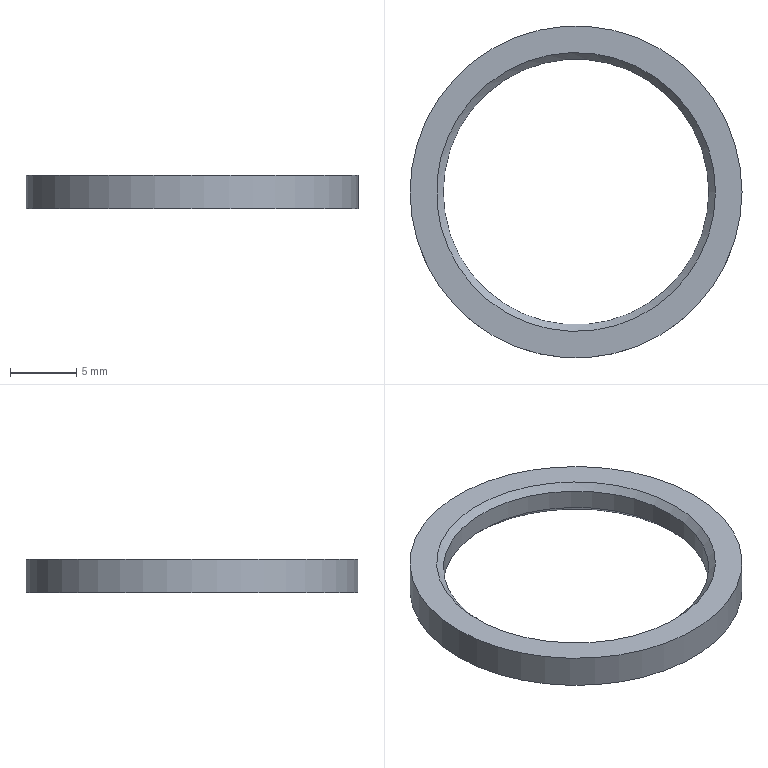Part | NX | features BREP 1 | 1 solid | 6 faces | box 25 x 25 x 2.5 mm | volume 425.817 mm3 | cone 2 | cylinder 2 | plane 2 | commonest cylinder face diameters 20 x1 25 x1
STEP:
#1=CARTESIAN_POINT('',(10.5,0.,0.));
#2=VERTEX_POINT('',#1);
#3=CARTESIAN_POINT('',(0.,0.,0.));
#4=DIRECTION('',(0.,0.,1.));
#5=DIRECTION('',(1.,0.,0.));
#6=AXIS2_PLACEMENT_3D('',#3,#4,#5);
#7=CIRCLE('',#6,10.5);
#8=EDGE_CURVE('',#2,#2,#7,.T.);
#9=ORIENTED_EDGE('',*,*,#8,.F.);
#10=EDGE_LOOP('',(#9));
#11=FACE_BOUND('',#10,.T.);
#12=CARTESIAN_POINT('',(10.,0.,0.5));
#13=VERTEX_POINT('',#12);
#14=CARTESIAN_POINT('',(0.,0.,0.5));
#15=DIRECTION('',(0.,0.,-1.));
#16=DIRECTION('',(1.,0.,0.));
#17=AXIS2_PLACEMENT_3D('',#14,#15,#16);
#18=CIRCLE('',#17,10.);
#19=EDGE_CURVE('',#13,#13,#18,.T.);
#20=ORIENTED_EDGE('',*,*,#19,.F.);
#21=EDGE_LOOP('',(#20));
#22=FACE_BOUND('',#21,.T.);
#23=CARTESIAN_POINT('',(0.,0.,0.));
#24=DIRECTION('',(0.,0.,-1.));
#25=DIRECTION('',(-1.,0.,0.));
#26=AXIS2_PLACEMENT_3D('',#23,#24,#25);
#27=CONICAL_SURFACE('',#26,10.5,0.7854);
#28=ADVANCED_FACE('',(#11,#22),#27,.F.);
#29=CARTESIAN_POINT('',(10.5,0.,2.5));
#30=VERTEX_POINT('',#29);
#31=CARTESIAN_POINT('',(0.,0.,2.5));
#32=DIRECTION('',(0.,0.,-1.));
#33=DIRECTION('',(1.,0.,0.));
#34=AXIS2_PLACEMENT_3D('',#31,#32,#33);
#35=CIRCLE('',#34,10.5);
#36=EDGE_CURVE('',#30,#30,#35,.T.);
#37=ORIENTED_EDGE('',*,*,#36,.F.);
#38=EDGE_LOOP('',(#37));
#39=FACE_BOUND('',#38,.T.);
#40=CARTESIAN_POINT('',(10.,0.,2.));
#41=VERTEX_POINT('',#40);
#42=CARTESIAN_POINT('',(0.,0.,2.));
#43=DIRECTION('',(0.,0.,1.));
#44=DIRECTION('',(1.,0.,0.));
#45=AXIS2_PLACEMENT_3D('',#42,#43,#44);
#46=CIRCLE('',#45,10.);
#47=EDGE_CURVE('',#41,#41,#46,.T.);
#48=ORIENTED_EDGE('',*,*,#47,.F.);
#49=EDGE_LOOP('',(#48));
#50=FACE_BOUND('',#49,.T.);
#51=CARTESIAN_POINT('',(0.,0.,2.));
#52=DIRECTION('',(0.,0.,1.));
#53=DIRECTION('',(1.,0.,0.));
#54=AXIS2_PLACEMENT_3D('',#51,#52,#53);
#55=CONICAL_SURFACE('',#54,10.,0.7854);
#56=ADVANCED_FACE('',(#39,#50),#55,.F.);
#57=ORIENTED_EDGE('',*,*,#19,.T.);
#58=EDGE_LOOP('',(#57));
#59=FACE_BOUND('',#58,.T.);
#60=ORIENTED_EDGE('',*,*,#47,.T.);
#61=EDGE_LOOP('',(#60));
#62=FACE_BOUND('',#61,.T.);
#63=CARTESIAN_POINT('',(0.,0.,2.5));
#64=DIRECTION('',(0.,0.,-1.));
#65=DIRECTION('',(-1.,0.,0.));
#66=AXIS2_PLACEMENT_3D('',#63,#64,#65);
#67=CYLINDRICAL_SURFACE('',#66,10.);
#68=ADVANCED_FACE('',(#59,#62),#67,.F.);
#69=CARTESIAN_POINT('',(12.5,0.,0.));
#70=VERTEX_POINT('',#69);
#71=CARTESIAN_POINT('',(0.,0.,0.));
#72=DIRECTION('',(0.,0.,1.));
#73=DIRECTION('',(1.,0.,0.));
#74=AXIS2_PLACEMENT_3D('',#71,#72,#73);
#75=CIRCLE('',#74,12.5);
#76=EDGE_CURVE('',#70,#70,#75,.T.);
#77=ORIENTED_EDGE('',*,*,#76,.T.);
#78=EDGE_LOOP('',(#77));
#79=FACE_BOUND('',#78,.T.);
#80=CARTESIAN_POINT('',(12.5,0.,2.5));
#81=VERTEX_POINT('',#80);
#82=CARTESIAN_POINT('',(0.,0.,2.5));
#83=DIRECTION('',(0.,0.,1.));
#84=DIRECTION('',(1.,0.,0.));
#85=AXIS2_PLACEMENT_3D('',#82,#83,#84);
#86=CIRCLE('',#85,12.5);
#87=EDGE_CURVE('',#81,#81,#86,.T.);
#88=ORIENTED_EDGE('',*,*,#87,.F.);
#89=EDGE_LOOP('',(#88));
#90=FACE_BOUND('',#89,.T.);
#91=CARTESIAN_POINT('',(0.,0.,2.5));
#92=DIRECTION('',(0.,0.,-1.));
#93=DIRECTION('',(-1.,0.,0.));
#94=AXIS2_PLACEMENT_3D('',#91,#92,#93);
#95=CYLINDRICAL_SURFACE('',#94,12.5);
#96=ADVANCED_FACE('',(#79,#90),#95,.T.);
#97=ORIENTED_EDGE('',*,*,#36,.T.);
#98=EDGE_LOOP('',(#97));
#99=FACE_BOUND('',#98,.T.);
#100=ORIENTED_EDGE('',*,*,#87,.T.);
#101=EDGE_LOOP('',(#100));
#102=FACE_BOUND('',#101,.T.);
#103=CARTESIAN_POINT('',(0.,0.,2.5));
#104=DIRECTION('',(0.,0.,1.));
#105=DIRECTION('',(1.,0.,0.));
#106=AXIS2_PLACEMENT_3D('',#103,#104,#105);
#107=PLANE('',#106);
#108=ADVANCED_FACE('',(#99,#102),#107,.T.);
#109=ORIENTED_EDGE('',*,*,#8,.T.);
#110=EDGE_LOOP('',(#109));
#111=FACE_BOUND('',#110,.T.);
#112=ORIENTED_EDGE('',*,*,#76,.F.);
#113=EDGE_LOOP('',(#112));
#114=FACE_BOUND('',#113,.T.);
#115=CARTESIAN_POINT('',(0.,0.,0.));
#116=DIRECTION('',(0.,0.,1.));
#117=DIRECTION('',(1.,0.,0.));
#118=AXIS2_PLACEMENT_3D('',#115,#116,#117);
#119=PLANE('',#118);
#120=ADVANCED_FACE('',(#111,#114),#119,.F.);
#121=CLOSED_SHELL('',(#28,#56,#68,#96,#108,#120));
#122=MANIFOLD_SOLID_BREP('',#121);
#123=(LENGTH_UNIT()NAMED_UNIT(*)SI_UNIT(.MILLI.,.METRE.));
#124=UNCERTAINTY_MEASURE_WITH_UNIT(LENGTH_MEASURE(0.00001),#123,'','');
#125=(NAMED_UNIT(*)PLANE_ANGLE_UNIT()SI_UNIT($,.RADIAN.));
#126=(NAMED_UNIT(*)SI_UNIT($,.STERADIAN.)SOLID_ANGLE_UNIT());
#127=(GEOMETRIC_REPRESENTATION_CONTEXT(3)GLOBAL_UNCERTAINTY_ASSIGNED_CONTEXT((#124))GLOBAL_UNIT_ASSIGNED_CONTEXT((#123,#125,#126))REPRESENTATION_CONTEXT('',''));
#128=ADVANCED_BREP_SHAPE_REPRESENTATION('',(#122),#127);